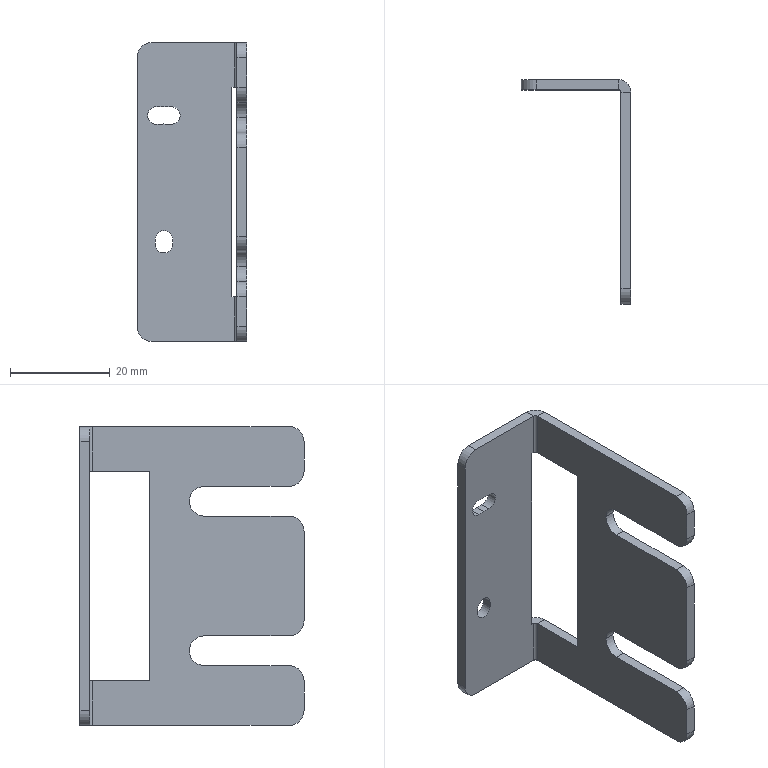Part | SolidWorks | features Fillet 2, ICE 2, Cut 1, ExtruThin 1, FlatPattern 1, FlattenBends 1, ProcessBends 1, SheetMetal 1 | 1 solid | 53 faces | box 22 x 45 x 60 mm | volume 5883 mm3 | plane 28 | cylinder 25 | commonest cylinder face diameters 6 x12 3.5 x5 1 x2 5 x2 47.3 x2 54.3 x2